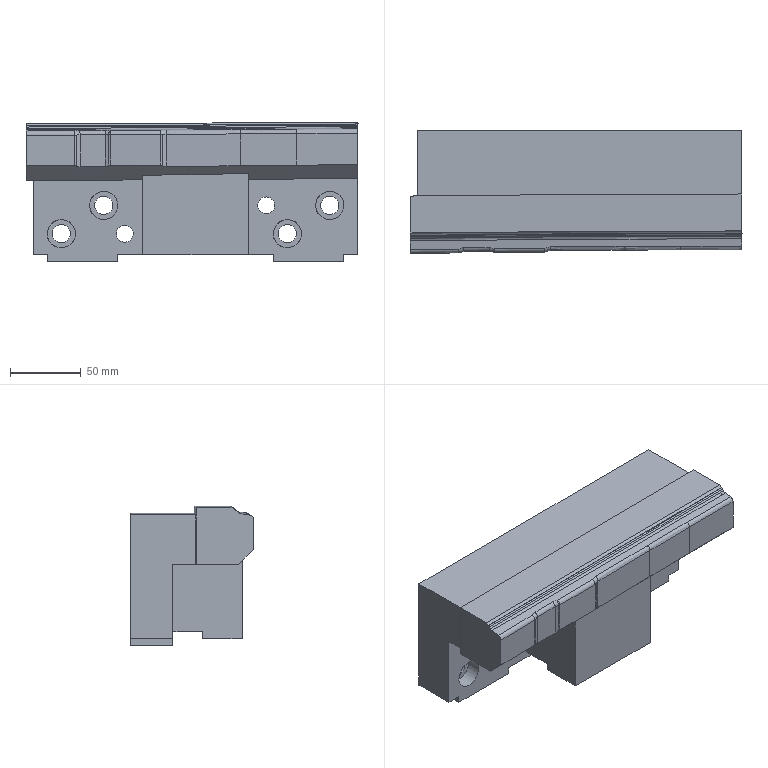Part | NX | features solid 2 | 1 solid | 68 faces | box 235 x 87.01 x 99.012 mm | volume 1257359 mm3 | spline 34 | plane 24 | cylinder 10 | commonest cylinder face diameters 13 x4 20 x4 12 x2